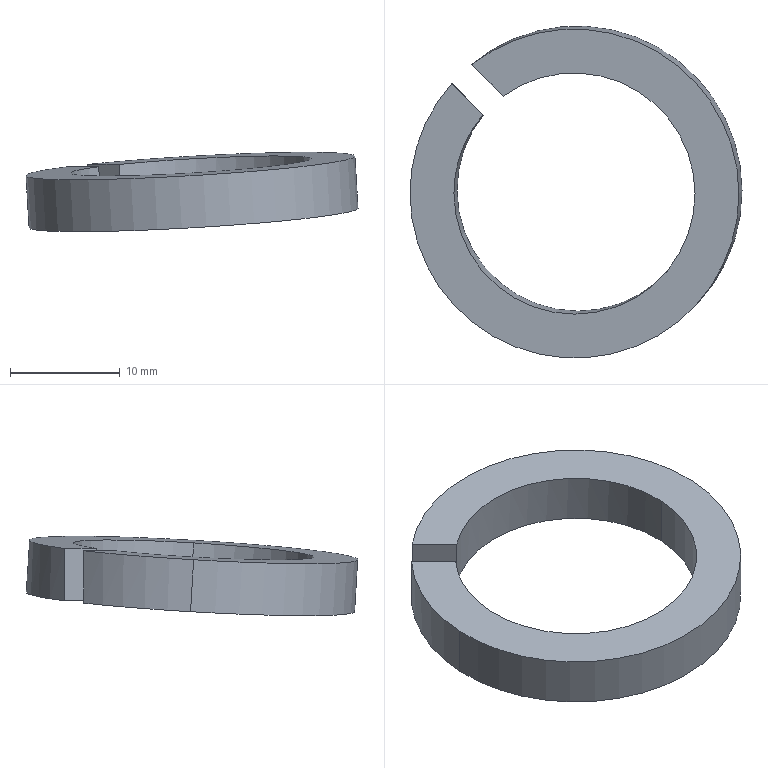Part | SolidWorks | features Boss 1, Cut 1, Extrusion 1, Helix 1, Sweep 1 | 1 solid | 10 faces | box 30.24 x 30.24 x 7.233 mm | volume 1507 mm3 | cylinder 6 | plane 4 | commonest cylinder face diameters 22 x3 30.013 x3
STEP:
#1=CARTESIAN_POINT('',(-11.46,9.692,0.3589));
#2=VERTEX_POINT('',#1);
#3=CARTESIAN_POINT('',(-15.007,-0.02719,-0.4249));
#4=VERTEX_POINT('',#3);
#5=CARTESIAN_POINT('',(-0.02719,-0.02719,0.4602));
#6=DIRECTION('',(-0.05888,-0.05888,0.9965));
#7=DIRECTION('',(0.9983,0.,0.05898));
#8=AXIS2_PLACEMENT_3D('',#5,#6,#7);
#9=CIRCLE('',#8,15.006);
#10=EDGE_CURVE('',#2,#4,#9,.T.);
#11=ORIENTED_EDGE('',*,*,#10,.T.);
#12=CARTESIAN_POINT('',(-15.287,-0.3069,4.309));
#13=VERTEX_POINT('',#12);
#14=CARTESIAN_POINT('',(-15.007,-0.02719,-0.4249));
#15=DIRECTION('',(-0.05888,-0.05888,0.9965));
#16=VECTOR('',#15,1000.);
#17=LINE('',#14,#16);
#18=EDGE_CURVE('',#4,#13,#17,.T.);
#19=ORIENTED_EDGE('',*,*,#18,.T.);
#20=CARTESIAN_POINT('',(-11.479,9.711,5.125));
#21=VERTEX_POINT('',#20);
#22=CARTESIAN_POINT('',(-0.3069,-0.3069,5.194));
#23=DIRECTION('',(-0.05888,-0.05888,0.9965));
#24=DIRECTION('',(0.9983,0.,0.05898));
#25=AXIS2_PLACEMENT_3D('',#22,#23,#24);
#26=CIRCLE('',#25,15.006);
#27=EDGE_CURVE('',#21,#13,#26,.T.);
#28=ORIENTED_EDGE('',*,*,#27,.F.);
#29=CARTESIAN_POINT('',(-11.46,9.692,0.3589));
#30=CARTESIAN_POINT('',(-11.468,9.7,1.946));
#31=CARTESIAN_POINT('',(-11.474,9.706,3.535));
#32=CARTESIAN_POINT('',(-11.479,9.711,5.125));
#33=(BOUNDED_CURVE()B_SPLINE_CURVE(3,(#29,#30,#31,#32),.UNSPECIFIED.,.F.,.F.)B_SPLINE_CURVE_WITH_KNOTS((4,4),(4.631,4.658),.UNSPECIFIED.)CURVE()GEOMETRIC_REPRESENTATION_ITEM()RATIONAL_B_SPLINE_CURVE((1.,0.9999,0.9999,1.))REPRESENTATION_ITEM(''));
#34=EDGE_CURVE('',#2,#21,#33,.T.);
#35=ORIENTED_EDGE('',*,*,#34,.F.);
#36=EDGE_LOOP('',(#11,#19,#28,#35));
#37=FACE_OUTER_BOUND('',#36,.T.);
#38=CARTESIAN_POINT('',(-0.02719,-0.02719,0.4602));
#39=DIRECTION('',(-0.05888,-0.05888,0.9965));
#40=DIRECTION('',(0.9983,0.,0.05898));
#41=AXIS2_PLACEMENT_3D('',#38,#39,#40);
#42=CYLINDRICAL_SURFACE('',#41,15.006);
#43=ADVANCED_FACE('',(#37),#42,.T.);
#44=ORIENTED_EDGE('',*,*,#18,.F.);
#45=CARTESIAN_POINT('',(14.953,-0.02719,1.345));
#46=VERTEX_POINT('',#45);
#47=CARTESIAN_POINT('',(-0.02719,-0.02719,0.4602));
#48=DIRECTION('',(-0.05888,-0.05888,0.9965));
#49=DIRECTION('',(0.9983,0.,0.05898));
#50=AXIS2_PLACEMENT_3D('',#47,#48,#49);
#51=CIRCLE('',#50,15.006);
#52=EDGE_CURVE('',#4,#46,#51,.T.);
#53=ORIENTED_EDGE('',*,*,#52,.T.);
#54=CARTESIAN_POINT('',(14.673,-0.3069,6.079));
#55=VERTEX_POINT('',#54);
#56=CARTESIAN_POINT('',(14.953,-0.02719,1.345));
#57=DIRECTION('',(-0.05888,-0.05888,0.9965));
#58=VECTOR('',#57,1000.);
#59=LINE('',#56,#58);
#60=EDGE_CURVE('',#46,#55,#59,.T.);
#61=ORIENTED_EDGE('',*,*,#60,.T.);
#62=CARTESIAN_POINT('',(-0.3069,-0.3069,5.194));
#63=DIRECTION('',(-0.05888,-0.05888,0.9965));
#64=DIRECTION('',(0.9983,0.,0.05898));
#65=AXIS2_PLACEMENT_3D('',#62,#63,#64);
#66=CIRCLE('',#65,15.006);
#67=EDGE_CURVE('',#13,#55,#66,.T.);
#68=ORIENTED_EDGE('',*,*,#67,.F.);
#69=EDGE_LOOP('',(#44,#53,#61,#68));
#70=FACE_OUTER_BOUND('',#69,.T.);
#71=CARTESIAN_POINT('',(-0.02719,-0.02719,0.4602));
#72=DIRECTION('',(-0.05888,-0.05888,0.9965));
#73=DIRECTION('',(0.9983,0.,0.05898));
#74=AXIS2_PLACEMENT_3D('',#71,#72,#73);
#75=CYLINDRICAL_SURFACE('',#74,15.006);
#76=ADVANCED_FACE('',(#70),#75,.T.);
#77=CARTESIAN_POINT('',(-11.008,-0.02719,-0.1886));
#78=VERTEX_POINT('',#77);
#79=CARTESIAN_POINT('',(10.954,-0.02719,1.109));
#80=VERTEX_POINT('',#79);
#81=CARTESIAN_POINT('',(-0.02719,-0.02719,0.4602));
#82=DIRECTION('',(-0.05888,-0.05888,0.9965));
#83=DIRECTION('',(0.9983,0.,0.05898));
#84=AXIS2_PLACEMENT_3D('',#81,#82,#83);
#85=CIRCLE('',#84,11.);
#86=EDGE_CURVE('',#78,#80,#85,.T.);
#87=ORIENTED_EDGE('',*,*,#86,.F.);
#88=CARTESIAN_POINT('',(-11.288,-0.3069,4.545));
#89=VERTEX_POINT('',#88);
#90=CARTESIAN_POINT('',(-11.008,-0.02719,-0.1886));
#91=DIRECTION('',(-0.05888,-0.05888,0.9965));
#92=VECTOR('',#91,1000.);
#93=LINE('',#90,#92);
#94=EDGE_CURVE('',#78,#89,#93,.T.);
#95=ORIENTED_EDGE('',*,*,#94,.T.);
#96=CARTESIAN_POINT('',(10.674,-0.3069,5.842));
#97=VERTEX_POINT('',#96);
#98=CARTESIAN_POINT('',(-0.3069,-0.3069,5.194));
#99=DIRECTION('',(-0.05888,-0.05888,0.9965));
#100=DIRECTION('',(0.9983,0.,0.05898));
#101=AXIS2_PLACEMENT_3D('',#98,#99,#100);
#102=CIRCLE('',#101,11.);
#103=EDGE_CURVE('',#89,#97,#102,.T.);
#104=ORIENTED_EDGE('',*,*,#103,.T.);
#105=CARTESIAN_POINT('',(10.954,-0.02719,1.109));
#106=DIRECTION('',(-0.05888,-0.05888,0.9965));
#107=VECTOR('',#106,1000.);
#108=LINE('',#105,#107);
#109=EDGE_CURVE('',#80,#97,#108,.T.);
#110=ORIENTED_EDGE('',*,*,#109,.F.);
#111=EDGE_LOOP('',(#87,#95,#104,#110));
#112=FACE_OUTER_BOUND('',#111,.T.);
#113=CARTESIAN_POINT('',(-0.02719,-0.02719,0.4602));
#114=DIRECTION('',(-0.05888,-0.05888,0.9965));
#115=DIRECTION('',(0.9983,0.,0.05898));
#116=AXIS2_PLACEMENT_3D('',#113,#114,#115);
#117=CYLINDRICAL_SURFACE('',#116,11.);
#118=ADVANCED_FACE('',(#112),#117,.F.);
#119=CARTESIAN_POINT('',(-6.84,8.608,0.5678));
#120=VERTEX_POINT('',#119);
#121=CARTESIAN_POINT('',(-0.02719,-0.02719,0.4602));
#122=DIRECTION('',(-0.05888,-0.05888,0.9965));
#123=DIRECTION('',(0.9983,0.,0.05898));
#124=AXIS2_PLACEMENT_3D('',#121,#122,#123);
#125=CIRCLE('',#124,11.);
#126=EDGE_CURVE('',#80,#120,#125,.T.);
#127=ORIENTED_EDGE('',*,*,#126,.F.);
#128=ORIENTED_EDGE('',*,*,#109,.T.);
#129=CARTESIAN_POINT('',(-6.802,8.57,5.334));
#130=VERTEX_POINT('',#129);
#131=CARTESIAN_POINT('',(-0.3069,-0.3069,5.194));
#132=DIRECTION('',(-0.05888,-0.05888,0.9965));
#133=DIRECTION('',(0.9983,0.,0.05898));
#134=AXIS2_PLACEMENT_3D('',#131,#132,#133);
#135=CIRCLE('',#134,11.);
#136=EDGE_CURVE('',#97,#130,#135,.T.);
#137=ORIENTED_EDGE('',*,*,#136,.T.);
#138=CARTESIAN_POINT('',(-6.802,8.57,5.334));
#139=CARTESIAN_POINT('',(-6.816,8.584,3.75));
#140=CARTESIAN_POINT('',(-6.829,8.597,2.161));
#141=CARTESIAN_POINT('',(-6.84,8.608,0.5678));
#142=(BOUNDED_CURVE()B_SPLINE_CURVE(3,(#138,#139,#140,#141),.UNSPECIFIED.,.F.,.F.)B_SPLINE_CURVE_WITH_KNOTS((4,4),(1.417,1.453),.UNSPECIFIED.)CURVE()GEOMETRIC_REPRESENTATION_ITEM()RATIONAL_B_SPLINE_CURVE((1.,0.9999,0.9999,1.))REPRESENTATION_ITEM(''));
#143=EDGE_CURVE('',#130,#120,#142,.T.);
#144=ORIENTED_EDGE('',*,*,#143,.T.);
#145=EDGE_LOOP('',(#127,#128,#137,#144));
#146=FACE_OUTER_BOUND('',#145,.T.);
#147=CARTESIAN_POINT('',(-0.02719,-0.02719,0.4602));
#148=DIRECTION('',(-0.05888,-0.05888,0.9965));
#149=DIRECTION('',(0.9983,0.,0.05898));
#150=AXIS2_PLACEMENT_3D('',#147,#148,#149);
#151=CYLINDRICAL_SURFACE('',#150,11.);
#152=ADVANCED_FACE('',(#146),#151,.F.);
#153=CARTESIAN_POINT('',(-8.64,6.873,5.125));
#154=VERTEX_POINT('',#153);
#155=CARTESIAN_POINT('',(-11.476,9.709,5.125));
#156=DIRECTION('',(0.7071,-0.7071,0.));
#157=VECTOR('',#156,1000.);
#158=LINE('',#155,#157);
#159=EDGE_CURVE('',#21,#154,#158,.T.);
#160=ORIENTED_EDGE('',*,*,#159,.F.);
#161=ORIENTED_EDGE('',*,*,#27,.T.);
#162=ORIENTED_EDGE('',*,*,#67,.T.);
#163=CARTESIAN_POINT('',(-9.66,11.428,5.334));
#164=VERTEX_POINT('',#163);
#165=CARTESIAN_POINT('',(-0.3069,-0.3069,5.194));
#166=DIRECTION('',(-0.05888,-0.05888,0.9965));
#167=DIRECTION('',(0.9983,0.,0.05898));
#168=AXIS2_PLACEMENT_3D('',#165,#166,#167);
#169=CIRCLE('',#168,15.006);
#170=EDGE_CURVE('',#55,#164,#169,.T.);
#171=ORIENTED_EDGE('',*,*,#170,.T.);
#172=CARTESIAN_POINT('',(-9.709,11.476,5.334));
#173=DIRECTION('',(-0.7071,0.7071,0.));
#174=VECTOR('',#173,1000.);
#175=LINE('',#172,#174);
#176=EDGE_CURVE('',#130,#164,#175,.T.);
#177=ORIENTED_EDGE('',*,*,#176,.F.);
#178=ORIENTED_EDGE('',*,*,#136,.F.);
#179=ORIENTED_EDGE('',*,*,#103,.F.);
#180=CARTESIAN_POINT('',(-0.3069,-0.3069,5.194));
#181=DIRECTION('',(-0.05888,-0.05888,0.9965));
#182=DIRECTION('',(0.9983,0.,0.05898));
#183=AXIS2_PLACEMENT_3D('',#180,#181,#182);
#184=CIRCLE('',#183,11.);
#185=EDGE_CURVE('',#154,#89,#184,.T.);
#186=ORIENTED_EDGE('',*,*,#185,.F.);
#187=EDGE_LOOP('',(#160,#161,#162,#171,#177,#178,#179,#186));
#188=FACE_OUTER_BOUND('',#187,.T.);
#189=CARTESIAN_POINT('',(-10.592,10.593,5.23));
#190=DIRECTION('',(-0.05888,-0.05888,0.9965));
#191=DIRECTION('',(0.9983,0.,0.05898));
#192=AXIS2_PLACEMENT_3D('',#189,#190,#191);
#193=PLANE('',#192);
#194=ADVANCED_FACE('',(#188),#193,.T.);
#195=ORIENTED_EDGE('',*,*,#94,.F.);
#196=CARTESIAN_POINT('',(-8.614,6.847,0.3589));
#197=VERTEX_POINT('',#196);
#198=CARTESIAN_POINT('',(-0.02719,-0.02719,0.4602));
#199=DIRECTION('',(-0.05888,-0.05888,0.9965));
#200=DIRECTION('',(0.9983,0.,0.05898));
#201=AXIS2_PLACEMENT_3D('',#198,#199,#200);
#202=CIRCLE('',#201,11.);
#203=EDGE_CURVE('',#197,#78,#202,.T.);
#204=ORIENTED_EDGE('',*,*,#203,.F.);
#205=CARTESIAN_POINT('',(-8.614,6.847,0.3589));
#206=CARTESIAN_POINT('',(-8.625,6.857,1.945));
#207=CARTESIAN_POINT('',(-8.633,6.866,3.534));
#208=CARTESIAN_POINT('',(-8.64,6.873,5.125));
#209=(BOUNDED_CURVE()B_SPLINE_CURVE(3,(#205,#206,#207,#208),.UNSPECIFIED.,.F.,.F.)B_SPLINE_CURVE_WITH_KNOTS((4,4),(4.602,4.638),.UNSPECIFIED.)CURVE()GEOMETRIC_REPRESENTATION_ITEM()RATIONAL_B_SPLINE_CURVE((1.,0.9999,0.9999,1.))REPRESENTATION_ITEM(''));
#210=EDGE_CURVE('',#197,#154,#209,.T.);
#211=ORIENTED_EDGE('',*,*,#210,.T.);
#212=ORIENTED_EDGE('',*,*,#185,.T.);
#213=EDGE_LOOP('',(#195,#204,#211,#212));
#214=FACE_OUTER_BOUND('',#213,.T.);
#215=CARTESIAN_POINT('',(-0.02719,-0.02719,0.4602));
#216=DIRECTION('',(-0.05888,-0.05888,0.9965));
#217=DIRECTION('',(0.9983,0.,0.05898));
#218=AXIS2_PLACEMENT_3D('',#215,#216,#217);
#219=CYLINDRICAL_SURFACE('',#218,11.);
#220=ADVANCED_FACE('',(#214),#219,.F.);
#221=ORIENTED_EDGE('',*,*,#60,.F.);
#222=CARTESIAN_POINT('',(-9.688,11.456,0.5678));
#223=VERTEX_POINT('',#222);
#224=CARTESIAN_POINT('',(-0.02719,-0.02719,0.4602));
#225=DIRECTION('',(-0.05888,-0.05888,0.9965));
#226=DIRECTION('',(0.9983,0.,0.05898));
#227=AXIS2_PLACEMENT_3D('',#224,#225,#226);
#228=CIRCLE('',#227,15.006);
#229=EDGE_CURVE('',#46,#223,#228,.T.);
#230=ORIENTED_EDGE('',*,*,#229,.T.);
#231=CARTESIAN_POINT('',(-9.66,11.428,5.334));
#232=CARTESIAN_POINT('',(-9.67,11.438,3.748));
#233=CARTESIAN_POINT('',(-9.68,11.447,2.159));
#234=CARTESIAN_POINT('',(-9.688,11.456,0.5678));
#235=(BOUNDED_CURVE()B_SPLINE_CURVE(3,(#231,#232,#233,#234),.UNSPECIFIED.,.F.,.F.)B_SPLINE_CURVE_WITH_KNOTS((4,4),(1.458,1.485),.UNSPECIFIED.)CURVE()GEOMETRIC_REPRESENTATION_ITEM()RATIONAL_B_SPLINE_CURVE((1.,0.9999,0.9999,1.))REPRESENTATION_ITEM(''));
#236=EDGE_CURVE('',#164,#223,#235,.T.);
#237=ORIENTED_EDGE('',*,*,#236,.F.);
#238=ORIENTED_EDGE('',*,*,#170,.F.);
#239=EDGE_LOOP('',(#221,#230,#237,#238));
#240=FACE_OUTER_BOUND('',#239,.T.);
#241=CARTESIAN_POINT('',(-0.02719,-0.02719,0.4602));
#242=DIRECTION('',(-0.05888,-0.05888,0.9965));
#243=DIRECTION('',(0.9983,0.,0.05898));
#244=AXIS2_PLACEMENT_3D('',#241,#242,#243);
#245=CYLINDRICAL_SURFACE('',#244,15.006);
#246=ADVANCED_FACE('',(#240),#245,.T.);
#247=ORIENTED_EDGE('',*,*,#10,.F.);
#248=CARTESIAN_POINT('',(-0.8839,-0.8839,0.3589));
#249=DIRECTION('',(0.7071,-0.7071,0.));
#250=VECTOR('',#249,1000.);
#251=LINE('',#248,#250);
#252=EDGE_CURVE('',#2,#197,#251,.T.);
#253=ORIENTED_EDGE('',*,*,#252,.T.);
#254=ORIENTED_EDGE('',*,*,#203,.T.);
#255=ORIENTED_EDGE('',*,*,#86,.T.);
#256=ORIENTED_EDGE('',*,*,#126,.T.);
#257=CARTESIAN_POINT('',(0.8839,0.8839,0.5678));
#258=DIRECTION('',(-0.7071,0.7071,0.));
#259=VECTOR('',#258,1000.);
#260=LINE('',#257,#259);
#261=EDGE_CURVE('',#120,#223,#260,.T.);
#262=ORIENTED_EDGE('',*,*,#261,.T.);
#263=ORIENTED_EDGE('',*,*,#229,.F.);
#264=ORIENTED_EDGE('',*,*,#52,.F.);
#265=EDGE_LOOP('',(#247,#253,#254,#255,#256,#262,#263,#264));
#266=FACE_OUTER_BOUND('',#265,.T.);
#267=CARTESIAN_POINT('',(-0.02719,-0.02719,0.4602));
#268=DIRECTION('',(-0.05888,-0.05888,0.9965));
#269=DIRECTION('',(0.9983,0.,0.05898));
#270=AXIS2_PLACEMENT_3D('',#267,#268,#269);
#271=PLANE('',#270);
#272=ADVANCED_FACE('',(#266),#271,.F.);
#273=ORIENTED_EDGE('',*,*,#176,.T.);
#274=ORIENTED_EDGE('',*,*,#236,.T.);
#275=ORIENTED_EDGE('',*,*,#261,.F.);
#276=ORIENTED_EDGE('',*,*,#143,.F.);
#277=EDGE_LOOP('',(#273,#274,#275,#276));
#278=FACE_OUTER_BOUND('',#277,.T.);
#279=CARTESIAN_POINT('',(-34.367,36.135,-0.7894));
#280=DIRECTION('',(0.7071,0.7071,0.));
#281=DIRECTION('',(-0.7071,0.7071,0.));
#282=AXIS2_PLACEMENT_3D('',#279,#280,#281);
#283=PLANE('',#282);
#284=ADVANCED_FACE('',(#278),#283,.F.);
#285=ORIENTED_EDGE('',*,*,#159,.T.);
#286=ORIENTED_EDGE('',*,*,#210,.F.);
#287=ORIENTED_EDGE('',*,*,#252,.F.);
#288=ORIENTED_EDGE('',*,*,#34,.T.);
#289=EDGE_LOOP('',(#285,#286,#287,#288));
#290=FACE_OUTER_BOUND('',#289,.T.);
#291=CARTESIAN_POINT('',(-1.133,-0.6347,-0.7894));
#292=DIRECTION('',(-0.7071,-0.7071,0.));
#293=DIRECTION('',(0.7071,-0.7071,0.));
#294=AXIS2_PLACEMENT_3D('',#291,#292,#293);
#295=PLANE('',#294);
#296=ADVANCED_FACE('',(#290),#295,.F.);
#297=CLOSED_SHELL('',(#43,#76,#118,#152,#194,#220,#246,#272,#284,#296));
#298=MANIFOLD_SOLID_BREP('',#297);
#299=CARTESIAN_POINT('',(0.,0.,0.));
#300=DIRECTION('',(0.,0.,1.));
#301=DIRECTION('',(1.,0.,0.));
#302=AXIS2_PLACEMENT_3D('',#299,#300,#301);
#303=(LENGTH_UNIT()NAMED_UNIT(*)SI_UNIT(.MILLI.,.METRE.));
#304=UNCERTAINTY_MEASURE_WITH_UNIT(LENGTH_MEASURE(0.00001),#303,'','');
#305=(NAMED_UNIT(*)PLANE_ANGLE_UNIT()SI_UNIT($,.RADIAN.));
#306=(NAMED_UNIT(*)SI_UNIT($,.STERADIAN.)SOLID_ANGLE_UNIT());
#307=(GEOMETRIC_REPRESENTATION_CONTEXT(3)GLOBAL_UNCERTAINTY_ASSIGNED_CONTEXT((#304))GLOBAL_UNIT_ASSIGNED_CONTEXT((#303,#305,#306))REPRESENTATION_CONTEXT('',''));
#308=ADVANCED_BREP_SHAPE_REPRESENTATION('',(#298,#302),#307);